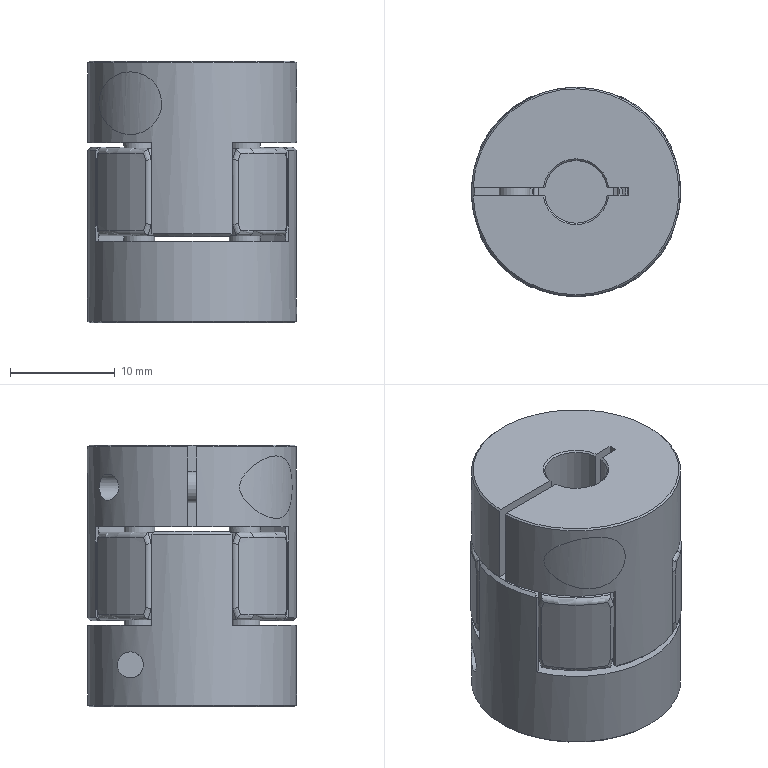Part | NX | features BREP 1 | 3 solids | 284 faces | box 20 x 20 x 25 mm | volume 6872 mm3 | cylinder 92 | plane 82 | spline 52 | cone 50 | torus 8 | commonest cylinder face diameters 22.846 x16 22.847 x16 0.4 x8 1 x8 2.997 x8 9.741 x8